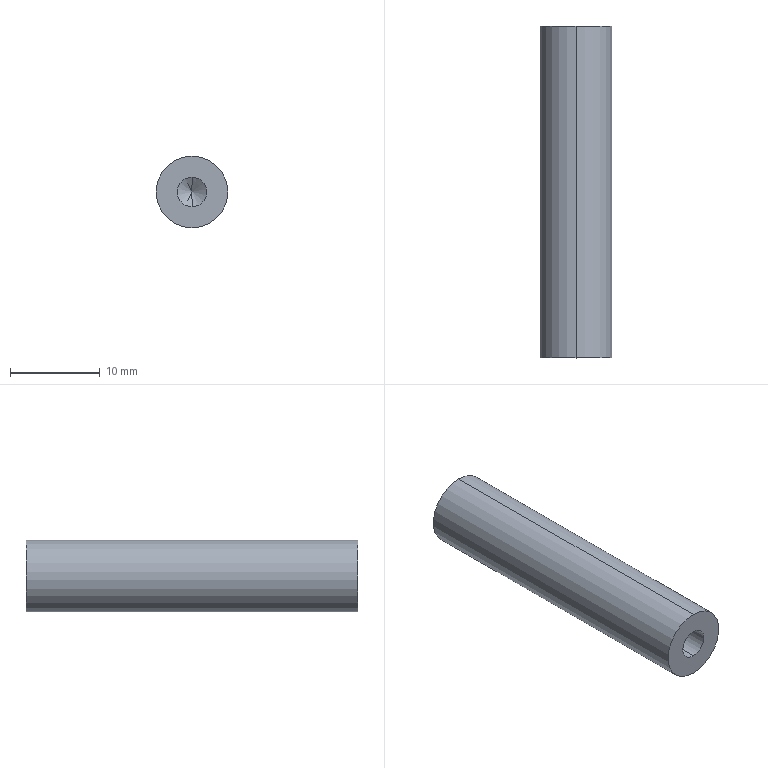Part | STEP file | connecting column | 1 solid | 12 faces | box 8 x 37 x 8 mm | volume 1657 mm3 | cylinder 6 | cone 4 | plane 2 | commonest cylinder face diameters 3.3 x4 8 x2
STEP:
#1=CARTESIAN_POINT('',(0.,0.,0.));
#2=DIRECTION('',(0.,0.,1.));
#3=DIRECTION('',(1.,0.,0.));
#4=AXIS2_PLACEMENT_3D('',#1,#2,#3);
#5=CARTESIAN_POINT('',(0.,25.5,1.65));
#6=VERTEX_POINT('',#5);
#7=CARTESIAN_POINT('',(0.,37.,1.65));
#8=VERTEX_POINT('',#7);
#9=CARTESIAN_POINT('',(0.,37.,1.65));
#10=DIRECTION('',(0.,1.,0.));
#11=VECTOR('',#10,1.);
#12=LINE('',#9,#11);
#13=CARTESIAN_POINT('',(0.,37.,0.));
#14=DIRECTION('',(0.,1.,0.));
#15=DIRECTION('',(0.,0.,1.));
#16=AXIS2_PLACEMENT_3D('',#13,#14,#15);
#17=CYLINDRICAL_SURFACE('',#16,1.65);
#18=CARTESIAN_POINT('',(6.283,0.));
#19=DIRECTION('',(0.,1.));
#20=VECTOR('',#19,1.);
#21=LINE('',#18,#20);
#22=(GEOMETRIC_REPRESENTATION_CONTEXT(2)PARAMETRIC_REPRESENTATION_CONTEXT()REPRESENTATION_CONTEXT('',''));
#23=DEFINITIONAL_REPRESENTATION('',(#21),#22);
#24=PCURVE('',#17,#23);
#25=CARTESIAN_POINT('',(0.,37.,0.));
#26=DIRECTION('',(0.,1.,0.));
#27=DIRECTION('',(0.,0.,1.));
#28=AXIS2_PLACEMENT_3D('',#25,#26,#27);
#29=CYLINDRICAL_SURFACE('',#28,1.65);
#30=CARTESIAN_POINT('',(0.,0.));
#31=DIRECTION('',(0.,1.));
#32=VECTOR('',#31,1.);
#33=LINE('',#30,#32);
#34=(GEOMETRIC_REPRESENTATION_CONTEXT(2)PARAMETRIC_REPRESENTATION_CONTEXT()REPRESENTATION_CONTEXT('',''));
#35=DEFINITIONAL_REPRESENTATION('',(#33),#34);
#36=PCURVE('',#29,#35);
#37=SURFACE_CURVE('',#12,(#24,#36),.PCURVE_S1.);
#38=EDGE_CURVE('',#6,#8,#37,.T.);
#39=ORIENTED_EDGE('',*,*,#38,.T.);
#40=CARTESIAN_POINT('',(0.,37.,-1.65));
#41=VERTEX_POINT('',#40);
#42=CARTESIAN_POINT('',(0.,37.,0.));
#43=DIRECTION('',(0.,1.,0.));
#44=DIRECTION('',(0.,0.,1.));
#45=AXIS2_PLACEMENT_3D('',#42,#43,#44);
#46=CIRCLE('',#45,1.65);
#47=CARTESIAN_POINT('',(0.,0.));
#48=DIRECTION('',(1.,0.));
#49=VECTOR('',#48,1.);
#50=LINE('',#47,#49);
#51=(GEOMETRIC_REPRESENTATION_CONTEXT(2)PARAMETRIC_REPRESENTATION_CONTEXT()REPRESENTATION_CONTEXT('',''));
#52=DEFINITIONAL_REPRESENTATION('',(#50),#51);
#53=PCURVE('',#17,#52);
#54=CARTESIAN_POINT('',(0.,37.,0.));
#55=DIRECTION('',(0.,1.,0.));
#56=DIRECTION('',(0.,0.,1.));
#57=AXIS2_PLACEMENT_3D('',#54,#55,#56);
#58=PLANE('',#57);
#59=CARTESIAN_POINT('',(0.,0.));
#60=DIRECTION('',(1.,0.));
#61=AXIS2_PLACEMENT_2D('',#59,#60);
#62=CIRCLE('',#61,1.65);
#63=(GEOMETRIC_REPRESENTATION_CONTEXT(2)PARAMETRIC_REPRESENTATION_CONTEXT()REPRESENTATION_CONTEXT('',''));
#64=DEFINITIONAL_REPRESENTATION('',(#62),#63);
#65=PCURVE('',#58,#64);
#66=SURFACE_CURVE('',#46,(#53,#65),.PCURVE_S1.);
#67=EDGE_CURVE('',#41,#8,#66,.T.);
#68=ORIENTED_EDGE('',*,*,#67,.F.);
#69=CARTESIAN_POINT('',(0.,25.5,-1.65));
#70=VERTEX_POINT('',#69);
#71=CARTESIAN_POINT('',(0.,37.,-1.65));
#72=DIRECTION('',(0.,1.,0.));
#73=VECTOR('',#72,1.);
#74=LINE('',#71,#73);
#75=CARTESIAN_POINT('',(3.142,0.));
#76=DIRECTION('',(0.,1.));
#77=VECTOR('',#76,1.);
#78=LINE('',#75,#77);
#79=(GEOMETRIC_REPRESENTATION_CONTEXT(2)PARAMETRIC_REPRESENTATION_CONTEXT()REPRESENTATION_CONTEXT('',''));
#80=DEFINITIONAL_REPRESENTATION('',(#78),#79);
#81=PCURVE('',#17,#80);
#82=CARTESIAN_POINT('',(3.142,0.));
#83=DIRECTION('',(0.,1.));
#84=VECTOR('',#83,1.);
#85=LINE('',#82,#84);
#86=(GEOMETRIC_REPRESENTATION_CONTEXT(2)PARAMETRIC_REPRESENTATION_CONTEXT()REPRESENTATION_CONTEXT('',''));
#87=DEFINITIONAL_REPRESENTATION('',(#85),#86);
#88=PCURVE('',#29,#87);
#89=SURFACE_CURVE('',#74,(#81,#88),.PCURVE_S1.);
#90=EDGE_CURVE('',#70,#41,#89,.T.);
#91=ORIENTED_EDGE('',*,*,#90,.F.);
#92=CARTESIAN_POINT('',(0.,25.5,0.));
#93=DIRECTION('',(0.,1.,0.));
#94=DIRECTION('',(0.,0.,1.));
#95=AXIS2_PLACEMENT_3D('',#92,#93,#94);
#96=CIRCLE('',#95,1.65);
#97=CARTESIAN_POINT('',(0.,-11.5));
#98=DIRECTION('',(1.,0.));
#99=VECTOR('',#98,1.);
#100=LINE('',#97,#99);
#101=(GEOMETRIC_REPRESENTATION_CONTEXT(2)PARAMETRIC_REPRESENTATION_CONTEXT()REPRESENTATION_CONTEXT('',''));
#102=DEFINITIONAL_REPRESENTATION('',(#100),#101);
#103=PCURVE('',#17,#102);
#104=CARTESIAN_POINT('',(0.,25.5,0.));
#105=DIRECTION('',(0.,1.,0.));
#106=DIRECTION('',(0.,0.,1.));
#107=AXIS2_PLACEMENT_3D('',#104,#105,#106);
#108=CONICAL_SURFACE('',#107,1.65,1.03);
#109=CARTESIAN_POINT('',(0.,0.));
#110=DIRECTION('',(1.,0.));
#111=VECTOR('',#110,1.);
#112=LINE('',#109,#111);
#113=(GEOMETRIC_REPRESENTATION_CONTEXT(2)PARAMETRIC_REPRESENTATION_CONTEXT()REPRESENTATION_CONTEXT('',''));
#114=DEFINITIONAL_REPRESENTATION('',(#112),#113);
#115=PCURVE('',#108,#114);
#116=SURFACE_CURVE('',#96,(#103,#115),.PCURVE_S1.);
#117=EDGE_CURVE('',#70,#6,#116,.T.);
#118=ORIENTED_EDGE('',*,*,#117,.T.);
#119=EDGE_LOOP('',(#39,#68,#91,#118));
#120=FACE_BOUND('',#119,.F.);
#121=ADVANCED_FACE('',(#120),#17,.F.);
#122=ORIENTED_EDGE('',*,*,#117,.F.);
#123=CARTESIAN_POINT('',(0.,24.509,0.));
#124=VERTEX_POINT('',#123);
#125=CARTESIAN_POINT('',(0.,25.5,-1.65));
#126=DIRECTION('',(0.,0.515,-0.8572));
#127=VECTOR('',#126,1.);
#128=LINE('',#125,#127);
#129=CARTESIAN_POINT('',(3.142,0.));
#130=DIRECTION('',(0.,1.));
#131=VECTOR('',#130,1.);
#132=LINE('',#129,#131);
#133=(GEOMETRIC_REPRESENTATION_CONTEXT(2)PARAMETRIC_REPRESENTATION_CONTEXT()REPRESENTATION_CONTEXT('',''));
#134=DEFINITIONAL_REPRESENTATION('',(#132),#133);
#135=PCURVE('',#108,#134);
#136=CARTESIAN_POINT('',(0.,25.5,0.));
#137=DIRECTION('',(0.,1.,0.));
#138=DIRECTION('',(0.,0.,1.));
#139=AXIS2_PLACEMENT_3D('',#136,#137,#138);
#140=CONICAL_SURFACE('',#139,1.65,1.03);
#141=CARTESIAN_POINT('',(3.142,0.));
#142=DIRECTION('',(0.,1.));
#143=VECTOR('',#142,1.);
#144=LINE('',#141,#143);
#145=(GEOMETRIC_REPRESENTATION_CONTEXT(2)PARAMETRIC_REPRESENTATION_CONTEXT()REPRESENTATION_CONTEXT('',''));
#146=DEFINITIONAL_REPRESENTATION('',(#144),#145);
#147=PCURVE('',#140,#146);
#148=SURFACE_CURVE('',#128,(#135,#147),.PCURVE_S1.);
#149=EDGE_CURVE('',#124,#70,#148,.T.);
#150=ORIENTED_EDGE('',*,*,#149,.F.);
#151=CARTESIAN_POINT('',(0.,25.5,1.65));
#152=DIRECTION('',(0.,0.515,0.8572));
#153=VECTOR('',#152,1.);
#154=LINE('',#151,#153);
#155=CARTESIAN_POINT('',(6.283,0.));
#156=DIRECTION('',(0.,1.));
#157=VECTOR('',#156,1.);
#158=LINE('',#155,#157);
#159=(GEOMETRIC_REPRESENTATION_CONTEXT(2)PARAMETRIC_REPRESENTATION_CONTEXT()REPRESENTATION_CONTEXT('',''));
#160=DEFINITIONAL_REPRESENTATION('',(#158),#159);
#161=PCURVE('',#108,#160);
#162=CARTESIAN_POINT('',(0.,0.));
#163=DIRECTION('',(0.,1.));
#164=VECTOR('',#163,1.);
#165=LINE('',#162,#164);
#166=(GEOMETRIC_REPRESENTATION_CONTEXT(2)PARAMETRIC_REPRESENTATION_CONTEXT()REPRESENTATION_CONTEXT('',''));
#167=DEFINITIONAL_REPRESENTATION('',(#165),#166);
#168=PCURVE('',#140,#167);
#169=SURFACE_CURVE('',#154,(#161,#168),.PCURVE_S1.);
#170=EDGE_CURVE('',#124,#6,#169,.T.);
#171=ORIENTED_EDGE('',*,*,#170,.T.);
#172=EDGE_LOOP('',(#122,#150,#171));
#173=FACE_BOUND('',#172,.F.);
#174=ADVANCED_FACE('',(#173),#108,.F.);
#175=CARTESIAN_POINT('',(0.,11.5,-1.65));
#176=VERTEX_POINT('',#175);
#177=CARTESIAN_POINT('',(0.,0.,-1.65));
#178=VERTEX_POINT('',#177);
#179=CARTESIAN_POINT('',(0.,0.,-1.65));
#180=DIRECTION('',(0.,-1.,0.));
#181=VECTOR('',#180,1.);
#182=LINE('',#179,#181);
#183=CARTESIAN_POINT('',(0.,0.,0.));
#184=DIRECTION('',(0.,-1.,0.));
#185=DIRECTION('',(0.,0.,-1.));
#186=AXIS2_PLACEMENT_3D('',#183,#184,#185);
#187=CYLINDRICAL_SURFACE('',#186,1.65);
#188=CARTESIAN_POINT('',(6.283,0.));
#189=DIRECTION('',(0.,1.));
#190=VECTOR('',#189,1.);
#191=LINE('',#188,#190);
#192=(GEOMETRIC_REPRESENTATION_CONTEXT(2)PARAMETRIC_REPRESENTATION_CONTEXT()REPRESENTATION_CONTEXT('',''));
#193=DEFINITIONAL_REPRESENTATION('',(#191),#192);
#194=PCURVE('',#187,#193);
#195=CARTESIAN_POINT('',(0.,0.,0.));
#196=DIRECTION('',(0.,-1.,0.));
#197=DIRECTION('',(0.,0.,-1.));
#198=AXIS2_PLACEMENT_3D('',#195,#196,#197);
#199=CYLINDRICAL_SURFACE('',#198,1.65);
#200=CARTESIAN_POINT('',(0.,0.));
#201=DIRECTION('',(0.,1.));
#202=VECTOR('',#201,1.);
#203=LINE('',#200,#202);
#204=(GEOMETRIC_REPRESENTATION_CONTEXT(2)PARAMETRIC_REPRESENTATION_CONTEXT()REPRESENTATION_CONTEXT('',''));
#205=DEFINITIONAL_REPRESENTATION('',(#203),#204);
#206=PCURVE('',#199,#205);
#207=SURFACE_CURVE('',#182,(#194,#206),.PCURVE_S1.);
#208=EDGE_CURVE('',#176,#178,#207,.T.);
#209=ORIENTED_EDGE('',*,*,#208,.T.);
#210=CARTESIAN_POINT('',(0.,0.,1.65));
#211=VERTEX_POINT('',#210);
#212=CARTESIAN_POINT('',(0.,0.,0.));
#213=DIRECTION('',(0.,-1.,0.));
#214=DIRECTION('',(0.,0.,-1.));
#215=AXIS2_PLACEMENT_3D('',#212,#213,#214);
#216=CIRCLE('',#215,1.65);
#217=CARTESIAN_POINT('',(0.,0.));
#218=DIRECTION('',(1.,0.));
#219=VECTOR('',#218,1.);
#220=LINE('',#217,#219);
#221=(GEOMETRIC_REPRESENTATION_CONTEXT(2)PARAMETRIC_REPRESENTATION_CONTEXT()REPRESENTATION_CONTEXT('',''));
#222=DEFINITIONAL_REPRESENTATION('',(#220),#221);
#223=PCURVE('',#187,#222);
#224=CARTESIAN_POINT('',(0.,0.,0.));
#225=DIRECTION('',(0.,1.,0.));
#226=DIRECTION('',(0.,0.,1.));
#227=AXIS2_PLACEMENT_3D('',#224,#225,#226);
#228=PLANE('',#227);
#229=CARTESIAN_POINT('',(-1.65,0.));
#230=CARTESIAN_POINT('',(-1.65,2.858));
#231=CARTESIAN_POINT('',(0.825,1.429));
#232=CARTESIAN_POINT('',(3.3,0.));
#233=CARTESIAN_POINT('',(0.825,-1.429));
#234=CARTESIAN_POINT('',(-1.65,-2.858));
#235=CARTESIAN_POINT('',(-1.65,0.));
#236=(BOUNDED_CURVE()B_SPLINE_CURVE(2,(#229,#230,#231,#232,#233,#234,#235),.UNSPECIFIED.,.T.,.F.)B_SPLINE_CURVE_WITH_KNOTS((1,2,2,2,2,1),(-2.094,0.,2.094,4.189,6.283,8.378),.UNSPECIFIED.)CURVE()GEOMETRIC_REPRESENTATION_ITEM()RATIONAL_B_SPLINE_CURVE((1.,0.5,1.,0.5,1.,0.5,1.))REPRESENTATION_ITEM(''));
#237=(GEOMETRIC_REPRESENTATION_CONTEXT(2)PARAMETRIC_REPRESENTATION_CONTEXT()REPRESENTATION_CONTEXT('',''));
#238=DEFINITIONAL_REPRESENTATION('',(#236),#237);
#239=PCURVE('',#228,#238);
#240=SURFACE_CURVE('',#216,(#223,#239),.PCURVE_S1.);
#241=EDGE_CURVE('',#211,#178,#240,.T.);
#242=ORIENTED_EDGE('',*,*,#241,.F.);
#243=CARTESIAN_POINT('',(0.,11.5,1.65));
#244=VERTEX_POINT('',#243);
#245=CARTESIAN_POINT('',(0.,0.,1.65));
#246=DIRECTION('',(0.,-1.,0.));
#247=VECTOR('',#246,1.);
#248=LINE('',#245,#247);
#249=CARTESIAN_POINT('',(3.142,0.));
#250=DIRECTION('',(0.,1.));
#251=VECTOR('',#250,1.);
#252=LINE('',#249,#251);
#253=(GEOMETRIC_REPRESENTATION_CONTEXT(2)PARAMETRIC_REPRESENTATION_CONTEXT()REPRESENTATION_CONTEXT('',''));
#254=DEFINITIONAL_REPRESENTATION('',(#252),#253);
#255=PCURVE('',#187,#254);
#256=CARTESIAN_POINT('',(3.142,0.));
#257=DIRECTION('',(0.,1.));
#258=VECTOR('',#257,1.);
#259=LINE('',#256,#258);
#260=(GEOMETRIC_REPRESENTATION_CONTEXT(2)PARAMETRIC_REPRESENTATION_CONTEXT()REPRESENTATION_CONTEXT('',''));
#261=DEFINITIONAL_REPRESENTATION('',(#259),#260);
#262=PCURVE('',#199,#261);
#263=SURFACE_CURVE('',#248,(#255,#262),.PCURVE_S1.);
#264=EDGE_CURVE('',#244,#211,#263,.T.);
#265=ORIENTED_EDGE('',*,*,#264,.F.);
#266=CARTESIAN_POINT('',(0.,11.5,0.));
#267=DIRECTION('',(0.,-1.,0.));
#268=DIRECTION('',(0.,0.,-1.));
#269=AXIS2_PLACEMENT_3D('',#266,#267,#268);
#270=CIRCLE('',#269,1.65);
#271=CARTESIAN_POINT('',(0.,-11.5));
#272=DIRECTION('',(1.,0.));
#273=VECTOR('',#272,1.);
#274=LINE('',#271,#273);
#275=(GEOMETRIC_REPRESENTATION_CONTEXT(2)PARAMETRIC_REPRESENTATION_CONTEXT()REPRESENTATION_CONTEXT('',''));
#276=DEFINITIONAL_REPRESENTATION('',(#274),#275);
#277=PCURVE('',#187,#276);
#278=CARTESIAN_POINT('',(0.,11.5,0.));
#279=DIRECTION('',(0.,-1.,0.));
#280=DIRECTION('',(0.,0.,-1.));
#281=AXIS2_PLACEMENT_3D('',#278,#279,#280);
#282=CONICAL_SURFACE('',#281,1.65,1.03);
#283=CARTESIAN_POINT('',(0.,0.));
#284=DIRECTION('',(1.,0.));
#285=VECTOR('',#284,1.);
#286=LINE('',#283,#285);
#287=(GEOMETRIC_REPRESENTATION_CONTEXT(2)PARAMETRIC_REPRESENTATION_CONTEXT()REPRESENTATION_CONTEXT('',''));
#288=DEFINITIONAL_REPRESENTATION('',(#286),#287);
#289=PCURVE('',#282,#288);
#290=SURFACE_CURVE('',#270,(#277,#289),.PCURVE_S1.);
#291=EDGE_CURVE('',#244,#176,#290,.T.);
#292=ORIENTED_EDGE('',*,*,#291,.T.);
#293=EDGE_LOOP('',(#209,#242,#265,#292));
#294=FACE_BOUND('',#293,.F.);
#295=ADVANCED_FACE('',(#294),#187,.F.);
#296=ORIENTED_EDGE('',*,*,#291,.F.);
#297=CARTESIAN_POINT('',(0.,12.491,0.));
#298=VERTEX_POINT('',#297);
#299=CARTESIAN_POINT('',(0.,11.5,1.65));
#300=DIRECTION('',(0.,-0.515,0.8572));
#301=VECTOR('',#300,1.);
#302=LINE('',#299,#301);
#303=CARTESIAN_POINT('',(3.142,0.));
#304=DIRECTION('',(0.,1.));
#305=VECTOR('',#304,1.);
#306=LINE('',#303,#305);
#307=(GEOMETRIC_REPRESENTATION_CONTEXT(2)PARAMETRIC_REPRESENTATION_CONTEXT()REPRESENTATION_CONTEXT('',''));
#308=DEFINITIONAL_REPRESENTATION('',(#306),#307);
#309=PCURVE('',#282,#308);
#310=CARTESIAN_POINT('',(0.,11.5,0.));
#311=DIRECTION('',(0.,-1.,0.));
#312=DIRECTION('',(0.,0.,-1.));
#313=AXIS2_PLACEMENT_3D('',#310,#311,#312);
#314=CONICAL_SURFACE('',#313,1.65,1.03);
#315=CARTESIAN_POINT('',(3.142,0.));
#316=DIRECTION('',(0.,1.));
#317=VECTOR('',#316,1.);
#318=LINE('',#315,#317);
#319=(GEOMETRIC_REPRESENTATION_CONTEXT(2)PARAMETRIC_REPRESENTATION_CONTEXT()REPRESENTATION_CONTEXT('',''));
#320=DEFINITIONAL_REPRESENTATION('',(#318),#319);
#321=PCURVE('',#314,#320);
#322=SURFACE_CURVE('',#302,(#309,#321),.PCURVE_S1.);
#323=EDGE_CURVE('',#298,#244,#322,.T.);
#324=ORIENTED_EDGE('',*,*,#323,.F.);
#325=CARTESIAN_POINT('',(0.,11.5,-1.65));
#326=DIRECTION('',(0.,-0.515,-0.8572));
#327=VECTOR('',#326,1.);
#328=LINE('',#325,#327);
#329=CARTESIAN_POINT('',(6.283,0.));
#330=DIRECTION('',(0.,1.));
#331=VECTOR('',#330,1.);
#332=LINE('',#329,#331);
#333=(GEOMETRIC_REPRESENTATION_CONTEXT(2)PARAMETRIC_REPRESENTATION_CONTEXT()REPRESENTATION_CONTEXT('',''));
#334=DEFINITIONAL_REPRESENTATION('',(#332),#333);
#335=PCURVE('',#282,#334);
#336=CARTESIAN_POINT('',(0.,0.));
#337=DIRECTION('',(0.,1.));
#338=VECTOR('',#337,1.);
#339=LINE('',#336,#338);
#340=(GEOMETRIC_REPRESENTATION_CONTEXT(2)PARAMETRIC_REPRESENTATION_CONTEXT()REPRESENTATION_CONTEXT('',''));
#341=DEFINITIONAL_REPRESENTATION('',(#339),#340);
#342=PCURVE('',#314,#341);
#343=SURFACE_CURVE('',#328,(#335,#342),.PCURVE_S1.);
#344=EDGE_CURVE('',#298,#176,#343,.T.);
#345=ORIENTED_EDGE('',*,*,#344,.T.);
#346=EDGE_LOOP('',(#296,#324,#345));
#347=FACE_BOUND('',#346,.F.);
#348=ADVANCED_FACE('',(#347),#282,.F.);
#349=CARTESIAN_POINT('',(0.,37.,4.));
#350=VERTEX_POINT('',#349);
#351=CARTESIAN_POINT('',(0.,37.,-4.));
#352=VERTEX_POINT('',#351);
#353=CARTESIAN_POINT('',(0.,37.,0.));
#354=DIRECTION('',(0.,1.,0.));
#355=DIRECTION('',(0.,0.,1.));
#356=AXIS2_PLACEMENT_3D('',#353,#354,#355);
#357=CIRCLE('',#356,4.);
#358=CARTESIAN_POINT('',(0.,37.,0.));
#359=DIRECTION('',(0.,-1.,0.));
#360=DIRECTION('',(0.,0.,-1.));
#361=AXIS2_PLACEMENT_3D('',#358,#359,#360);
#362=CYLINDRICAL_SURFACE('',#361,4.);
#363=CARTESIAN_POINT('',(3.142,0.));
#364=DIRECTION('',(-1.,0.));
#365=VECTOR('',#364,1.);
#366=LINE('',#363,#365);
#367=(GEOMETRIC_REPRESENTATION_CONTEXT(2)PARAMETRIC_REPRESENTATION_CONTEXT()REPRESENTATION_CONTEXT('',''));
#368=DEFINITIONAL_REPRESENTATION('',(#366),#367);
#369=PCURVE('',#362,#368);
#370=CARTESIAN_POINT('',(0.,0.));
#371=DIRECTION('',(1.,0.));
#372=AXIS2_PLACEMENT_2D('',#370,#371);
#373=CIRCLE('',#372,4.);
#374=(GEOMETRIC_REPRESENTATION_CONTEXT(2)PARAMETRIC_REPRESENTATION_CONTEXT()REPRESENTATION_CONTEXT('',''));
#375=DEFINITIONAL_REPRESENTATION('',(#373),#374);
#376=PCURVE('',#58,#375);
#377=SURFACE_CURVE('',#357,(#369,#376),.PCURVE_S1.);
#378=EDGE_CURVE('',#350,#352,#377,.T.);
#379=ORIENTED_EDGE('',*,*,#378,.F.);
#380=CARTESIAN_POINT('',(0.,0.,4.));
#381=VERTEX_POINT('',#380);
#382=CARTESIAN_POINT('',(0.,37.,4.));
#383=DIRECTION('',(0.,-1.,0.));
#384=VECTOR('',#383,1.);
#385=LINE('',#382,#384);
#386=CARTESIAN_POINT('',(3.142,0.));
#387=DIRECTION('',(0.,1.));
#388=VECTOR('',#387,1.);
#389=LINE('',#386,#388);
#390=(GEOMETRIC_REPRESENTATION_CONTEXT(2)PARAMETRIC_REPRESENTATION_CONTEXT()REPRESENTATION_CONTEXT('',''));
#391=DEFINITIONAL_REPRESENTATION('',(#389),#390);
#392=PCURVE('',#362,#391);
#393=CARTESIAN_POINT('',(0.,37.,0.));
#394=DIRECTION('',(0.,-1.,0.));
#395=DIRECTION('',(0.,0.,-1.));
#396=AXIS2_PLACEMENT_3D('',#393,#394,#395);
#397=CYLINDRICAL_SURFACE('',#396,4.);
#398=CARTESIAN_POINT('',(3.142,0.));
#399=DIRECTION('',(0.,1.));
#400=VECTOR('',#399,1.);
#401=LINE('',#398,#400);
#402=(GEOMETRIC_REPRESENTATION_CONTEXT(2)PARAMETRIC_REPRESENTATION_CONTEXT()REPRESENTATION_CONTEXT('',''));
#403=DEFINITIONAL_REPRESENTATION('',(#401),#402);
#404=PCURVE('',#397,#403);
#405=SURFACE_CURVE('',#385,(#392,#404),.PCURVE_S1.);
#406=EDGE_CURVE('',#350,#381,#405,.T.);
#407=ORIENTED_EDGE('',*,*,#406,.T.);
#408=CARTESIAN_POINT('',(0.,0.,-4.));
#409=VERTEX_POINT('',#408);
#410=CARTESIAN_POINT('',(0.,0.,0.));
#411=DIRECTION('',(0.,1.,0.));
#412=DIRECTION('',(0.,0.,1.));
#413=AXIS2_PLACEMENT_3D('',#410,#411,#412);
#414=CIRCLE('',#413,4.);
#415=CARTESIAN_POINT('',(3.142,37.));
#416=DIRECTION('',(-1.,0.));
#417=VECTOR('',#416,1.);
#418=LINE('',#415,#417);
#419=(GEOMETRIC_REPRESENTATION_CONTEXT(2)PARAMETRIC_REPRESENTATION_CONTEXT()REPRESENTATION_CONTEXT('',''));
#420=DEFINITIONAL_REPRESENTATION('',(#418),#419);
#421=PCURVE('',#362,#420);
#422=CARTESIAN_POINT('',(0.,0.));
#423=DIRECTION('',(1.,0.));
#424=AXIS2_PLACEMENT_2D('',#422,#423);
#425=CIRCLE('',#424,4.);
#426=(GEOMETRIC_REPRESENTATION_CONTEXT(2)PARAMETRIC_REPRESENTATION_CONTEXT()REPRESENTATION_CONTEXT('',''));
#427=DEFINITIONAL_REPRESENTATION('',(#425),#426);
#428=PCURVE('',#228,#427);
#429=SURFACE_CURVE('',#414,(#421,#428),.PCURVE_S1.);
#430=EDGE_CURVE('',#381,#409,#429,.T.);
#431=ORIENTED_EDGE('',*,*,#430,.T.);
#432=CARTESIAN_POINT('',(0.,37.,-4.));
#433=DIRECTION('',(0.,-1.,0.));
#434=VECTOR('',#433,1.);
#435=LINE('',#432,#434);
#436=CARTESIAN_POINT('',(0.,0.));
#437=DIRECTION('',(0.,1.));
#438=VECTOR('',#437,1.);
#439=LINE('',#436,#438);
#440=(GEOMETRIC_REPRESENTATION_CONTEXT(2)PARAMETRIC_REPRESENTATION_CONTEXT()REPRESENTATION_CONTEXT('',''));
#441=DEFINITIONAL_REPRESENTATION('',(#439),#440);
#442=PCURVE('',#362,#441);
#443=CARTESIAN_POINT('',(6.283,0.));
#444=DIRECTION('',(0.,1.));
#445=VECTOR('',#444,1.);
#446=LINE('',#443,#445);
#447=(GEOMETRIC_REPRESENTATION_CONTEXT(2)PARAMETRIC_REPRESENTATION_CONTEXT()REPRESENTATION_CONTEXT('',''));
#448=DEFINITIONAL_REPRESENTATION('',(#446),#447);
#449=PCURVE('',#397,#448);
#450=SURFACE_CURVE('',#435,(#442,#449),.PCURVE_S1.);
#451=EDGE_CURVE('',#352,#409,#450,.T.);
#452=ORIENTED_EDGE('',*,*,#451,.F.);
#453=EDGE_LOOP('',(#379,#407,#431,#452));
#454=FACE_BOUND('',#453,.T.);
#455=ADVANCED_FACE('',(#454),#362,.T.);
#456=ORIENTED_EDGE('',*,*,#406,.F.);
#457=CARTESIAN_POINT('',(0.,37.,0.));
#458=DIRECTION('',(0.,1.,0.));
#459=DIRECTION('',(0.,0.,1.));
#460=AXIS2_PLACEMENT_3D('',#457,#458,#459);
#461=CIRCLE('',#460,4.);
#462=CARTESIAN_POINT('',(9.425,0.));
#463=DIRECTION('',(-1.,0.));
#464=VECTOR('',#463,1.);
#465=LINE('',#462,#464);
#466=(GEOMETRIC_REPRESENTATION_CONTEXT(2)PARAMETRIC_REPRESENTATION_CONTEXT()REPRESENTATION_CONTEXT('',''));
#467=DEFINITIONAL_REPRESENTATION('',(#465),#466);
#468=PCURVE('',#397,#467);
#469=CARTESIAN_POINT('',(0.,0.));
#470=DIRECTION('',(1.,0.));
#471=AXIS2_PLACEMENT_2D('',#469,#470);
#472=CIRCLE('',#471,4.);
#473=(GEOMETRIC_REPRESENTATION_CONTEXT(2)PARAMETRIC_REPRESENTATION_CONTEXT()REPRESENTATION_CONTEXT('',''));
#474=DEFINITIONAL_REPRESENTATION('',(#472),#473);
#475=PCURVE('',#58,#474);
#476=SURFACE_CURVE('',#461,(#468,#475),.PCURVE_S1.);
#477=EDGE_CURVE('',#352,#350,#476,.T.);
#478=ORIENTED_EDGE('',*,*,#477,.F.);
#479=ORIENTED_EDGE('',*,*,#451,.T.);
#480=CARTESIAN_POINT('',(0.,0.,0.));
#481=DIRECTION('',(0.,1.,0.));
#482=DIRECTION('',(0.,0.,1.));
#483=AXIS2_PLACEMENT_3D('',#480,#481,#482);
#484=CIRCLE('',#483,4.);
#485=CARTESIAN_POINT('',(9.425,37.));
#486=DIRECTION('',(-1.,0.));
#487=VECTOR('',#486,1.);
#488=LINE('',#485,#487);
#489=(GEOMETRIC_REPRESENTATION_CONTEXT(2)PARAMETRIC_REPRESENTATION_CONTEXT()REPRESENTATION_CONTEXT('',''));
#490=DEFINITIONAL_REPRESENTATION('',(#488),#489);
#491=PCURVE('',#397,#490);
#492=CARTESIAN_POINT('',(0.,0.));
#493=DIRECTION('',(1.,0.));
#494=AXIS2_PLACEMENT_2D('',#492,#493);
#495=CIRCLE('',#494,4.);
#496=(GEOMETRIC_REPRESENTATION_CONTEXT(2)PARAMETRIC_REPRESENTATION_CONTEXT()REPRESENTATION_CONTEXT('',''));
#497=DEFINITIONAL_REPRESENTATION('',(#495),#496);
#498=PCURVE('',#228,#497);
#499=SURFACE_CURVE('',#484,(#491,#498),.PCURVE_S1.);
#500=EDGE_CURVE('',#409,#381,#499,.T.);
#501=ORIENTED_EDGE('',*,*,#500,.T.);
#502=EDGE_LOOP('',(#456,#478,#479,#501));
#503=FACE_BOUND('',#502,.T.);
#504=ADVANCED_FACE('',(#503),#397,.T.);
#505=CARTESIAN_POINT('',(0.,37.,0.));
#506=DIRECTION('',(0.,1.,0.));
#507=DIRECTION('',(0.,0.,1.));
#508=AXIS2_PLACEMENT_3D('',#505,#506,#507);
#509=CIRCLE('',#508,1.65);
#510=CARTESIAN_POINT('',(0.,0.));
#511=DIRECTION('',(1.,0.));
#512=AXIS2_PLACEMENT_2D('',#510,#511);
#513=CIRCLE('',#512,1.65);
#514=(GEOMETRIC_REPRESENTATION_CONTEXT(2)PARAMETRIC_REPRESENTATION_CONTEXT()REPRESENTATION_CONTEXT('',''));
#515=DEFINITIONAL_REPRESENTATION('',(#513),#514);
#516=PCURVE('',#58,#515);
#517=CARTESIAN_POINT('',(0.,0.));
#518=DIRECTION('',(1.,0.));
#519=VECTOR('',#518,1.);
#520=LINE('',#517,#519);
#521=(GEOMETRIC_REPRESENTATION_CONTEXT(2)PARAMETRIC_REPRESENTATION_CONTEXT()REPRESENTATION_CONTEXT('',''));
#522=DEFINITIONAL_REPRESENTATION('',(#520),#521);
#523=PCURVE('',#29,#522);
#524=SURFACE_CURVE('',#509,(#516,#523),.PCURVE_S1.);
#525=EDGE_CURVE('',#8,#41,#524,.T.);
#526=ORIENTED_EDGE('',*,*,#525,.F.);
#527=ORIENTED_EDGE('',*,*,#67,.F.);
#528=EDGE_LOOP('',(#526,#527));
#529=FACE_BOUND('',#528,.T.);
#530=ORIENTED_EDGE('',*,*,#477,.T.);
#531=ORIENTED_EDGE('',*,*,#378,.T.);
#532=EDGE_LOOP('',(#530,#531));
#533=FACE_BOUND('',#532,.T.);
#534=ADVANCED_FACE('',(#529,#533),#58,.T.);
#535=CARTESIAN_POINT('',(0.,0.,0.));
#536=DIRECTION('',(0.,-1.,0.));
#537=DIRECTION('',(0.,0.,-1.));
#538=AXIS2_PLACEMENT_3D('',#535,#536,#537);
#539=CIRCLE('',#538,1.65);
#540=CARTESIAN_POINT('',(-1.65,0.));
#541=CARTESIAN_POINT('',(-1.65,2.858));
#542=CARTESIAN_POINT('',(0.825,1.429));
#543=CARTESIAN_POINT('',(3.3,0.));
#544=CARTESIAN_POINT('',(0.825,-1.429));
#545=CARTESIAN_POINT('',(-1.65,-2.858));
#546=CARTESIAN_POINT('',(-1.65,0.));
#547=(BOUNDED_CURVE()B_SPLINE_CURVE(2,(#540,#541,#542,#543,#544,#545,#546),.UNSPECIFIED.,.T.,.F.)B_SPLINE_CURVE_WITH_KNOTS((1,2,2,2,2,1),(-2.094,0.,2.094,4.189,6.283,8.378),.UNSPECIFIED.)CURVE()GEOMETRIC_REPRESENTATION_ITEM()RATIONAL_B_SPLINE_CURVE((1.,0.5,1.,0.5,1.,0.5,1.))REPRESENTATION_ITEM(''));
#548=(GEOMETRIC_REPRESENTATION_CONTEXT(2)PARAMETRIC_REPRESENTATION_CONTEXT()REPRESENTATION_CONTEXT('',''));
#549=DEFINITIONAL_REPRESENTATION('',(#547),#548);
#550=PCURVE('',#228,#549);
#551=CARTESIAN_POINT('',(0.,0.));
#552=DIRECTION('',(1.,0.));
#553=VECTOR('',#552,1.);
#554=LINE('',#551,#553);
#555=(GEOMETRIC_REPRESENTATION_CONTEXT(2)PARAMETRIC_REPRESENTATION_CONTEXT()REPRESENTATION_CONTEXT('',''));
#556=DEFINITIONAL_REPRESENTATION('',(#554),#555);
#557=PCURVE('',#199,#556);
#558=SURFACE_CURVE('',#539,(#550,#557),.PCURVE_S1.);
#559=EDGE_CURVE('',#178,#211,#558,.T.);
#560=ORIENTED_EDGE('',*,*,#559,.F.);
#561=ORIENTED_EDGE('',*,*,#241,.F.);
#562=EDGE_LOOP('',(#560,#561));
#563=FACE_BOUND('',#562,.T.);
#564=ORIENTED_EDGE('',*,*,#500,.F.);
#565=ORIENTED_EDGE('',*,*,#430,.F.);
#566=EDGE_LOOP('',(#564,#565));
#567=FACE_BOUND('',#566,.T.);
#568=ADVANCED_FACE('',(#563,#567),#228,.F.);
#569=CARTESIAN_POINT('',(0.,11.5,0.));
#570=DIRECTION('',(0.,-1.,0.));
#571=DIRECTION('',(0.,0.,-1.));
#572=AXIS2_PLACEMENT_3D('',#569,#570,#571);
#573=CIRCLE('',#572,1.65);
#574=CARTESIAN_POINT('',(0.,0.));
#575=DIRECTION('',(1.,0.));
#576=VECTOR('',#575,1.);
#577=LINE('',#574,#576);
#578=(GEOMETRIC_REPRESENTATION_CONTEXT(2)PARAMETRIC_REPRESENTATION_CONTEXT()REPRESENTATION_CONTEXT('',''));
#579=DEFINITIONAL_REPRESENTATION('',(#577),#578);
#580=PCURVE('',#314,#579);
#581=CARTESIAN_POINT('',(0.,-11.5));
#582=DIRECTION('',(1.,0.));
#583=VECTOR('',#582,1.);
#584=LINE('',#581,#583);
#585=(GEOMETRIC_REPRESENTATION_CONTEXT(2)PARAMETRIC_REPRESENTATION_CONTEXT()REPRESENTATION_CONTEXT('',''));
#586=DEFINITIONAL_REPRESENTATION('',(#584),#585);
#587=PCURVE('',#199,#586);
#588=SURFACE_CURVE('',#573,(#580,#587),.PCURVE_S1.);
#589=EDGE_CURVE('',#176,#244,#588,.T.);
#590=ORIENTED_EDGE('',*,*,#589,.F.);
#591=ORIENTED_EDGE('',*,*,#344,.F.);
#592=ORIENTED_EDGE('',*,*,#323,.T.);
#593=EDGE_LOOP('',(#590,#591,#592));
#594=FACE_BOUND('',#593,.F.);
#595=ADVANCED_FACE('',(#594),#314,.F.);
#596=ORIENTED_EDGE('',*,*,#559,.F.);
#597=ORIENTED_EDGE('',*,*,#208,.F.);
#598=ORIENTED_EDGE('',*,*,#589,.T.);
#599=ORIENTED_EDGE('',*,*,#264,.T.);
#600=EDGE_LOOP('',(#596,#597,#598,#599));
#601=FACE_BOUND('',#600,.F.);
#602=ADVANCED_FACE('',(#601),#199,.F.);
#603=CARTESIAN_POINT('',(0.,25.5,0.));
#604=DIRECTION('',(0.,1.,0.));
#605=DIRECTION('',(0.,0.,1.));
#606=AXIS2_PLACEMENT_3D('',#603,#604,#605);
#607=CIRCLE('',#606,1.65);
#608=CARTESIAN_POINT('',(0.,0.));
#609=DIRECTION('',(1.,0.));
#610=VECTOR('',#609,1.);
#611=LINE('',#608,#610);
#612=(GEOMETRIC_REPRESENTATION_CONTEXT(2)PARAMETRIC_REPRESENTATION_CONTEXT()REPRESENTATION_CONTEXT('',''));
#613=DEFINITIONAL_REPRESENTATION('',(#611),#612);
#614=PCURVE('',#140,#613);
#615=CARTESIAN_POINT('',(0.,-11.5));
#616=DIRECTION('',(1.,0.));
#617=VECTOR('',#616,1.);
#618=LINE('',#615,#617);
#619=(GEOMETRIC_REPRESENTATION_CONTEXT(2)PARAMETRIC_REPRESENTATION_CONTEXT()REPRESENTATION_CONTEXT('',''));
#620=DEFINITIONAL_REPRESENTATION('',(#618),#619);
#621=PCURVE('',#29,#620);
#622=SURFACE_CURVE('',#607,(#614,#621),.PCURVE_S1.);
#623=EDGE_CURVE('',#6,#70,#622,.T.);
#624=ORIENTED_EDGE('',*,*,#623,.F.);
#625=ORIENTED_EDGE('',*,*,#170,.F.);
#626=ORIENTED_EDGE('',*,*,#149,.T.);
#627=EDGE_LOOP('',(#624,#625,#626));
#628=FACE_BOUND('',#627,.F.);
#629=ADVANCED_FACE('',(#628),#140,.F.);
#630=ORIENTED_EDGE('',*,*,#525,.F.);
#631=ORIENTED_EDGE('',*,*,#38,.F.);
#632=ORIENTED_EDGE('',*,*,#623,.T.);
#633=ORIENTED_EDGE('',*,*,#90,.T.);
#634=EDGE_LOOP('',(#630,#631,#632,#633));
#635=FACE_BOUND('',#634,.F.);
#636=ADVANCED_FACE('',(#635),#29,.F.);
#637=CLOSED_SHELL('',(#121,#174,#295,#348,#455,#504,#534,#568,#595,#602,#629,#636));
#638=MANIFOLD_SOLID_BREP('',#637);
#639=(LENGTH_UNIT()NAMED_UNIT(*)SI_UNIT(.MILLI.,.METRE.));
#640=UNCERTAINTY_MEASURE_WITH_UNIT(LENGTH_MEASURE(0.0000001),#639,'','');
#641=(NAMED_UNIT(*)PLANE_ANGLE_UNIT()SI_UNIT($,.RADIAN.));
#642=(NAMED_UNIT(*)SI_UNIT($,.STERADIAN.)SOLID_ANGLE_UNIT());
#643=(GEOMETRIC_REPRESENTATION_CONTEXT(3)GLOBAL_UNCERTAINTY_ASSIGNED_CONTEXT((#640))GLOBAL_UNIT_ASSIGNED_CONTEXT((#639,#641,#642))REPRESENTATION_CONTEXT('',''));
#644=ADVANCED_BREP_SHAPE_REPRESENTATION('',(#4,#638),#643);